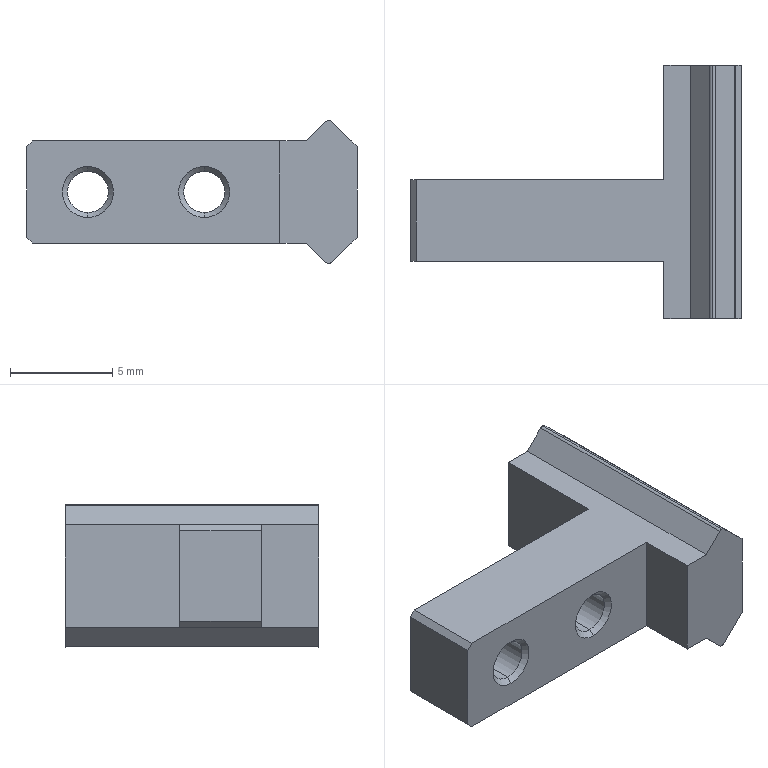Part | SolidWorks | features BaseBody 1 | 1 solid | 35 faces | box 16.2 x 12.4 x 6.994 mm | volume 484.765 mm3 | plane 20 | cone 8 | cylinder 7 | commonest cylinder face diameters 2.013 x4 0.4 x3
STEP:
#1=CARTESIAN_POINT('',(-42.341,-14.4,3.439));
#2=VERTEX_POINT('',#1);
#3=CARTESIAN_POINT('',(-42.2,-14.4,3.497));
#4=VERTEX_POINT('',#3);
#5=CARTESIAN_POINT('',(-42.2,-14.4,3.297));
#6=DIRECTION('',(0.,1.,0.));
#7=DIRECTION('',(1.,0.,0.));
#8=AXIS2_PLACEMENT_3D('',#5,#6,#7);
#9=CIRCLE('',#8,0.2);
#10=EDGE_CURVE('',#2,#4,#9,.T.);
#11=ORIENTED_EDGE('',*,*,#10,.T.);
#12=CARTESIAN_POINT('',(-42.2,-2.,3.497));
#13=VERTEX_POINT('',#12);
#14=CARTESIAN_POINT('',(-42.2,-14.4,3.497));
#15=DIRECTION('',(0.,1.,0.));
#16=VECTOR('',#15,1000.);
#17=LINE('',#14,#16);
#18=EDGE_CURVE('',#4,#13,#17,.T.);
#19=ORIENTED_EDGE('',*,*,#18,.T.);
#20=CARTESIAN_POINT('',(-42.341,-2.,3.439));
#21=VERTEX_POINT('',#20);
#22=CARTESIAN_POINT('',(-42.2,-2.,3.297));
#23=DIRECTION('',(0.,1.,0.));
#24=DIRECTION('',(1.,0.,0.));
#25=AXIS2_PLACEMENT_3D('',#22,#23,#24);
#26=CIRCLE('',#25,0.2);
#27=EDGE_CURVE('',#21,#13,#26,.T.);
#28=ORIENTED_EDGE('',*,*,#27,.F.);
#29=CARTESIAN_POINT('',(-42.341,-14.4,3.439));
#30=DIRECTION('',(0.,1.,0.));
#31=VECTOR('',#30,1000.);
#32=LINE('',#29,#31);
#33=EDGE_CURVE('',#2,#21,#32,.T.);
#34=ORIENTED_EDGE('',*,*,#33,.F.);
#35=EDGE_LOOP('',(#11,#19,#28,#34));
#36=FACE_OUTER_BOUND('',#35,.T.);
#37=CARTESIAN_POINT('',(-42.2,-14.4,3.297));
#38=DIRECTION('',(0.,1.,0.));
#39=DIRECTION('',(0.,0.,1.));
#40=AXIS2_PLACEMENT_3D('',#37,#38,#39);
#41=CYLINDRICAL_SURFACE('',#40,0.2);
#42=ADVANCED_FACE('',(#36),#41,.T.);
#43=CARTESIAN_POINT('',(-54.,-11.357,-1.006));
#44=VERTEX_POINT('',#43);
#45=CARTESIAN_POINT('',(-54.,-11.357,1.006));
#46=VERTEX_POINT('',#45);
#47=CARTESIAN_POINT('',(-54.,-11.357,0.));
#48=DIRECTION('',(0.,1.,0.));
#49=DIRECTION('',(0.,0.,1.));
#50=AXIS2_PLACEMENT_3D('',#47,#48,#49);
#51=CIRCLE('',#50,1.006);
#52=EDGE_CURVE('',#44,#46,#51,.T.);
#53=ORIENTED_EDGE('',*,*,#52,.T.);
#54=CARTESIAN_POINT('',(-54.,-11.6,1.25));
#55=VERTEX_POINT('',#54);
#56=CARTESIAN_POINT('',(-54.,-11.6,1.25));
#57=DIRECTION('',(0.,-0.7071,0.7071));
#58=VECTOR('',#57,1000.);
#59=LINE('',#56,#58);
#60=EDGE_CURVE('',#46,#55,#59,.T.);
#61=ORIENTED_EDGE('',*,*,#60,.T.);
#62=CARTESIAN_POINT('',(-54.,-11.6,-1.25));
#63=VERTEX_POINT('',#62);
#64=CARTESIAN_POINT('',(-54.,-11.6,0.));
#65=DIRECTION('',(0.,1.,0.));
#66=DIRECTION('',(0.,0.,1.));
#67=AXIS2_PLACEMENT_3D('',#64,#65,#66);
#68=CIRCLE('',#67,1.25);
#69=EDGE_CURVE('',#63,#55,#68,.T.);
#70=ORIENTED_EDGE('',*,*,#69,.F.);
#71=CARTESIAN_POINT('',(-54.,-11.6,-1.25));
#72=DIRECTION('',(0.,-0.7071,-0.7071));
#73=VECTOR('',#72,1000.);
#74=LINE('',#71,#73);
#75=EDGE_CURVE('',#44,#63,#74,.T.);
#76=ORIENTED_EDGE('',*,*,#75,.F.);
#77=EDGE_LOOP('',(#53,#61,#70,#76));
#78=FACE_OUTER_BOUND('',#77,.T.);
#79=CARTESIAN_POINT('',(-54.,-11.6,0.));
#80=DIRECTION('',(0.,-1.,0.));
#81=DIRECTION('',(0.,0.,-1.));
#82=AXIS2_PLACEMENT_3D('',#79,#80,#81);
#83=CONICAL_SURFACE('',#82,1.25,0.7854);
#84=ADVANCED_FACE('',(#78),#83,.F.);
#85=ORIENTED_EDGE('',*,*,#52,.F.);
#86=CARTESIAN_POINT('',(-54.,-7.833,-1.006));
#87=VERTEX_POINT('',#86);
#88=CARTESIAN_POINT('',(-54.,-7.59,-1.006));
#89=DIRECTION('',(0.,1.,0.));
#90=VECTOR('',#89,1000.);
#91=LINE('',#88,#90);
#92=EDGE_CURVE('',#44,#87,#91,.T.);
#93=ORIENTED_EDGE('',*,*,#92,.T.);
#94=CARTESIAN_POINT('',(-54.,-7.833,1.006));
#95=VERTEX_POINT('',#94);
#96=CARTESIAN_POINT('',(-54.,-7.833,0.));
#97=DIRECTION('',(0.,1.,0.));
#98=DIRECTION('',(0.,0.,1.));
#99=AXIS2_PLACEMENT_3D('',#96,#97,#98);
#100=CIRCLE('',#99,1.006);
#101=EDGE_CURVE('',#87,#95,#100,.T.);
#102=ORIENTED_EDGE('',*,*,#101,.T.);
#103=CARTESIAN_POINT('',(-54.,-7.59,1.006));
#104=DIRECTION('',(0.,1.,0.));
#105=VECTOR('',#104,1000.);
#106=LINE('',#103,#105);
#107=EDGE_CURVE('',#46,#95,#106,.T.);
#108=ORIENTED_EDGE('',*,*,#107,.F.);
#109=EDGE_LOOP('',(#85,#93,#102,#108));
#110=FACE_OUTER_BOUND('',#109,.T.);
#111=CARTESIAN_POINT('',(-54.,-7.59,0.));
#112=DIRECTION('',(0.,1.,0.));
#113=DIRECTION('',(0.,0.,1.));
#114=AXIS2_PLACEMENT_3D('',#111,#112,#113);
#115=CYLINDRICAL_SURFACE('',#114,1.006);
#116=ADVANCED_FACE('',(#110),#115,.F.);
#117=ORIENTED_EDGE('',*,*,#101,.F.);
#118=CARTESIAN_POINT('',(-54.,-7.6,-1.24));
#119=VERTEX_POINT('',#118);
#120=CARTESIAN_POINT('',(-54.,-7.833,-1.006));
#121=DIRECTION('',(0.,0.7071,-0.7071));
#122=VECTOR('',#121,1000.);
#123=LINE('',#120,#122);
#124=EDGE_CURVE('',#87,#119,#123,.T.);
#125=ORIENTED_EDGE('',*,*,#124,.T.);
#126=CARTESIAN_POINT('',(-54.,-7.6,1.24));
#127=VERTEX_POINT('',#126);
#128=CARTESIAN_POINT('',(-54.,-7.6,0.));
#129=DIRECTION('',(0.,-1.,0.));
#130=DIRECTION('',(0.,0.,1.));
#131=AXIS2_PLACEMENT_3D('',#128,#129,#130);
#132=CIRCLE('',#131,1.24);
#133=EDGE_CURVE('',#127,#119,#132,.T.);
#134=ORIENTED_EDGE('',*,*,#133,.F.);
#135=CARTESIAN_POINT('',(-54.,-7.833,1.006));
#136=DIRECTION('',(0.,0.7071,0.7071));
#137=VECTOR('',#136,1000.);
#138=LINE('',#135,#137);
#139=EDGE_CURVE('',#95,#127,#138,.T.);
#140=ORIENTED_EDGE('',*,*,#139,.F.);
#141=EDGE_LOOP('',(#117,#125,#134,#140));
#142=FACE_OUTER_BOUND('',#141,.T.);
#143=CARTESIAN_POINT('',(-54.,-7.833,0.));
#144=DIRECTION('',(0.,1.,0.));
#145=DIRECTION('',(0.,0.,1.));
#146=AXIS2_PLACEMENT_3D('',#143,#144,#145);
#147=CONICAL_SURFACE('',#146,1.006,0.7854);
#148=ADVANCED_FACE('',(#142),#147,.F.);
#149=CARTESIAN_POINT('',(-48.3,-11.357,-1.006));
#150=VERTEX_POINT('',#149);
#151=CARTESIAN_POINT('',(-48.3,-11.357,1.006));
#152=VERTEX_POINT('',#151);
#153=CARTESIAN_POINT('',(-48.3,-11.357,0.));
#154=DIRECTION('',(0.,1.,0.));
#155=DIRECTION('',(0.,0.,1.));
#156=AXIS2_PLACEMENT_3D('',#153,#154,#155);
#157=CIRCLE('',#156,1.006);
#158=EDGE_CURVE('',#150,#152,#157,.T.);
#159=ORIENTED_EDGE('',*,*,#158,.T.);
#160=CARTESIAN_POINT('',(-48.3,-11.6,1.25));
#161=VERTEX_POINT('',#160);
#162=CARTESIAN_POINT('',(-48.3,-11.6,1.25));
#163=DIRECTION('',(0.,-0.7071,0.7071));
#164=VECTOR('',#163,1000.);
#165=LINE('',#162,#164);
#166=EDGE_CURVE('',#152,#161,#165,.T.);
#167=ORIENTED_EDGE('',*,*,#166,.T.);
#168=CARTESIAN_POINT('',(-48.3,-11.6,-1.25));
#169=VERTEX_POINT('',#168);
#170=CARTESIAN_POINT('',(-48.3,-11.6,0.));
#171=DIRECTION('',(0.,1.,0.));
#172=DIRECTION('',(0.,0.,1.));
#173=AXIS2_PLACEMENT_3D('',#170,#171,#172);
#174=CIRCLE('',#173,1.25);
#175=EDGE_CURVE('',#169,#161,#174,.T.);
#176=ORIENTED_EDGE('',*,*,#175,.F.);
#177=CARTESIAN_POINT('',(-48.3,-11.6,-1.25));
#178=DIRECTION('',(0.,-0.7071,-0.7071));
#179=VECTOR('',#178,1000.);
#180=LINE('',#177,#179);
#181=EDGE_CURVE('',#150,#169,#180,.T.);
#182=ORIENTED_EDGE('',*,*,#181,.F.);
#183=EDGE_LOOP('',(#159,#167,#176,#182));
#184=FACE_OUTER_BOUND('',#183,.T.);
#185=CARTESIAN_POINT('',(-48.3,-11.6,0.));
#186=DIRECTION('',(0.,-1.,0.));
#187=DIRECTION('',(0.,0.,-1.));
#188=AXIS2_PLACEMENT_3D('',#185,#186,#187);
#189=CONICAL_SURFACE('',#188,1.25,0.7854);
#190=ADVANCED_FACE('',(#184),#189,.F.);
#191=ORIENTED_EDGE('',*,*,#158,.F.);
#192=CARTESIAN_POINT('',(-48.3,-7.833,-1.006));
#193=VERTEX_POINT('',#192);
#194=CARTESIAN_POINT('',(-48.3,-7.59,-1.006));
#195=DIRECTION('',(0.,1.,0.));
#196=VECTOR('',#195,1000.);
#197=LINE('',#194,#196);
#198=EDGE_CURVE('',#150,#193,#197,.T.);
#199=ORIENTED_EDGE('',*,*,#198,.T.);
#200=CARTESIAN_POINT('',(-48.3,-7.833,1.006));
#201=VERTEX_POINT('',#200);
#202=CARTESIAN_POINT('',(-48.3,-7.833,0.));
#203=DIRECTION('',(0.,1.,0.));
#204=DIRECTION('',(0.,0.,1.));
#205=AXIS2_PLACEMENT_3D('',#202,#203,#204);
#206=CIRCLE('',#205,1.006);
#207=EDGE_CURVE('',#193,#201,#206,.T.);
#208=ORIENTED_EDGE('',*,*,#207,.T.);
#209=CARTESIAN_POINT('',(-48.3,-7.59,1.006));
#210=DIRECTION('',(0.,1.,0.));
#211=VECTOR('',#210,1000.);
#212=LINE('',#209,#211);
#213=EDGE_CURVE('',#152,#201,#212,.T.);
#214=ORIENTED_EDGE('',*,*,#213,.F.);
#215=EDGE_LOOP('',(#191,#199,#208,#214));
#216=FACE_OUTER_BOUND('',#215,.T.);
#217=CARTESIAN_POINT('',(-48.3,-7.59,0.));
#218=DIRECTION('',(0.,1.,0.));
#219=DIRECTION('',(0.,0.,1.));
#220=AXIS2_PLACEMENT_3D('',#217,#218,#219);
#221=CYLINDRICAL_SURFACE('',#220,1.006);
#222=ADVANCED_FACE('',(#216),#221,.F.);
#223=ORIENTED_EDGE('',*,*,#207,.F.);
#224=CARTESIAN_POINT('',(-48.3,-7.6,-1.24));
#225=VERTEX_POINT('',#224);
#226=CARTESIAN_POINT('',(-48.3,-7.833,-1.006));
#227=DIRECTION('',(0.,0.7071,-0.7071));
#228=VECTOR('',#227,1000.);
#229=LINE('',#226,#228);
#230=EDGE_CURVE('',#193,#225,#229,.T.);
#231=ORIENTED_EDGE('',*,*,#230,.T.);
#232=CARTESIAN_POINT('',(-48.3,-7.6,1.24));
#233=VERTEX_POINT('',#232);
#234=CARTESIAN_POINT('',(-48.3,-7.6,0.));
#235=DIRECTION('',(0.,-1.,0.));
#236=DIRECTION('',(0.,0.,1.));
#237=AXIS2_PLACEMENT_3D('',#234,#235,#236);
#238=CIRCLE('',#237,1.24);
#239=EDGE_CURVE('',#233,#225,#238,.T.);
#240=ORIENTED_EDGE('',*,*,#239,.F.);
#241=CARTESIAN_POINT('',(-48.3,-7.833,1.006));
#242=DIRECTION('',(0.,0.7071,0.7071));
#243=VECTOR('',#242,1000.);
#244=LINE('',#241,#243);
#245=EDGE_CURVE('',#201,#233,#244,.T.);
#246=ORIENTED_EDGE('',*,*,#245,.F.);
#247=EDGE_LOOP('',(#223,#231,#240,#246));
#248=FACE_OUTER_BOUND('',#247,.T.);
#249=CARTESIAN_POINT('',(-48.3,-7.833,0.));
#250=DIRECTION('',(0.,1.,0.));
#251=DIRECTION('',(0.,0.,1.));
#252=AXIS2_PLACEMENT_3D('',#249,#250,#251);
#253=CONICAL_SURFACE('',#252,1.006,0.7854);
#254=ADVANCED_FACE('',(#248),#253,.F.);
#255=ORIENTED_EDGE('',*,*,#230,.F.);
#256=CARTESIAN_POINT('',(-48.3,-7.833,0.));
#257=DIRECTION('',(0.,1.,0.));
#258=DIRECTION('',(0.,0.,1.));
#259=AXIS2_PLACEMENT_3D('',#256,#257,#258);
#260=CIRCLE('',#259,1.006);
#261=EDGE_CURVE('',#201,#193,#260,.T.);
#262=ORIENTED_EDGE('',*,*,#261,.F.);
#263=ORIENTED_EDGE('',*,*,#245,.T.);
#264=CARTESIAN_POINT('',(-48.3,-7.6,0.));
#265=DIRECTION('',(0.,-1.,0.));
#266=DIRECTION('',(0.,0.,1.));
#267=AXIS2_PLACEMENT_3D('',#264,#265,#266);
#268=CIRCLE('',#267,1.24);
#269=EDGE_CURVE('',#225,#233,#268,.T.);
#270=ORIENTED_EDGE('',*,*,#269,.F.);
#271=EDGE_LOOP('',(#255,#262,#263,#270));
#272=FACE_OUTER_BOUND('',#271,.T.);
#273=CARTESIAN_POINT('',(-48.3,-7.833,0.));
#274=DIRECTION('',(0.,1.,0.));
#275=DIRECTION('',(0.,0.,1.));
#276=AXIS2_PLACEMENT_3D('',#273,#274,#275);
#277=CONICAL_SURFACE('',#276,1.006,0.7854);
#278=ADVANCED_FACE('',(#272),#277,.F.);
#279=ORIENTED_EDGE('',*,*,#198,.F.);
#280=CARTESIAN_POINT('',(-48.3,-11.357,0.));
#281=DIRECTION('',(0.,1.,0.));
#282=DIRECTION('',(0.,0.,1.));
#283=AXIS2_PLACEMENT_3D('',#280,#281,#282);
#284=CIRCLE('',#283,1.006);
#285=EDGE_CURVE('',#152,#150,#284,.T.);
#286=ORIENTED_EDGE('',*,*,#285,.F.);
#287=ORIENTED_EDGE('',*,*,#213,.T.);
#288=ORIENTED_EDGE('',*,*,#261,.T.);
#289=EDGE_LOOP('',(#279,#286,#287,#288));
#290=FACE_OUTER_BOUND('',#289,.T.);
#291=CARTESIAN_POINT('',(-48.3,-7.59,0.));
#292=DIRECTION('',(0.,1.,0.));
#293=DIRECTION('',(0.,0.,1.));
#294=AXIS2_PLACEMENT_3D('',#291,#292,#293);
#295=CYLINDRICAL_SURFACE('',#294,1.006);
#296=ADVANCED_FACE('',(#290),#295,.F.);
#297=ORIENTED_EDGE('',*,*,#166,.F.);
#298=ORIENTED_EDGE('',*,*,#285,.T.);
#299=ORIENTED_EDGE('',*,*,#181,.T.);
#300=CARTESIAN_POINT('',(-48.3,-11.6,0.));
#301=DIRECTION('',(0.,1.,0.));
#302=DIRECTION('',(0.,0.,1.));
#303=AXIS2_PLACEMENT_3D('',#300,#301,#302);
#304=CIRCLE('',#303,1.25);
#305=EDGE_CURVE('',#161,#169,#304,.T.);
#306=ORIENTED_EDGE('',*,*,#305,.F.);
#307=EDGE_LOOP('',(#297,#298,#299,#306));
#308=FACE_OUTER_BOUND('',#307,.T.);
#309=CARTESIAN_POINT('',(-48.3,-11.6,0.));
#310=DIRECTION('',(0.,-1.,0.));
#311=DIRECTION('',(0.,0.,-1.));
#312=AXIS2_PLACEMENT_3D('',#309,#310,#311);
#313=CONICAL_SURFACE('',#312,1.25,0.7854);
#314=ADVANCED_FACE('',(#308),#313,.F.);
#315=ORIENTED_EDGE('',*,*,#124,.F.);
#316=CARTESIAN_POINT('',(-54.,-7.833,0.));
#317=DIRECTION('',(0.,1.,0.));
#318=DIRECTION('',(0.,0.,1.));
#319=AXIS2_PLACEMENT_3D('',#316,#317,#318);
#320=CIRCLE('',#319,1.006);
#321=EDGE_CURVE('',#95,#87,#320,.T.);
#322=ORIENTED_EDGE('',*,*,#321,.F.);
#323=ORIENTED_EDGE('',*,*,#139,.T.);
#324=CARTESIAN_POINT('',(-54.,-7.6,0.));
#325=DIRECTION('',(0.,-1.,0.));
#326=DIRECTION('',(0.,0.,1.));
#327=AXIS2_PLACEMENT_3D('',#324,#325,#326);
#328=CIRCLE('',#327,1.24);
#329=EDGE_CURVE('',#119,#127,#328,.T.);
#330=ORIENTED_EDGE('',*,*,#329,.F.);
#331=EDGE_LOOP('',(#315,#322,#323,#330));
#332=FACE_OUTER_BOUND('',#331,.T.);
#333=CARTESIAN_POINT('',(-54.,-7.833,0.));
#334=DIRECTION('',(0.,1.,0.));
#335=DIRECTION('',(0.,0.,1.));
#336=AXIS2_PLACEMENT_3D('',#333,#334,#335);
#337=CONICAL_SURFACE('',#336,1.006,0.7854);
#338=ADVANCED_FACE('',(#332),#337,.F.);
#339=ORIENTED_EDGE('',*,*,#92,.F.);
#340=CARTESIAN_POINT('',(-54.,-11.357,0.));
#341=DIRECTION('',(0.,1.,0.));
#342=DIRECTION('',(0.,0.,1.));
#343=AXIS2_PLACEMENT_3D('',#340,#341,#342);
#344=CIRCLE('',#343,1.006);
#345=EDGE_CURVE('',#46,#44,#344,.T.);
#346=ORIENTED_EDGE('',*,*,#345,.F.);
#347=ORIENTED_EDGE('',*,*,#107,.T.);
#348=ORIENTED_EDGE('',*,*,#321,.T.);
#349=EDGE_LOOP('',(#339,#346,#347,#348));
#350=FACE_OUTER_BOUND('',#349,.T.);
#351=CARTESIAN_POINT('',(-54.,-7.59,0.));
#352=DIRECTION('',(0.,1.,0.));
#353=DIRECTION('',(0.,0.,1.));
#354=AXIS2_PLACEMENT_3D('',#351,#352,#353);
#355=CYLINDRICAL_SURFACE('',#354,1.006);
#356=ADVANCED_FACE('',(#350),#355,.F.);
#357=ORIENTED_EDGE('',*,*,#60,.F.);
#358=ORIENTED_EDGE('',*,*,#345,.T.);
#359=ORIENTED_EDGE('',*,*,#75,.T.);
#360=CARTESIAN_POINT('',(-54.,-11.6,0.));
#361=DIRECTION('',(0.,1.,0.));
#362=DIRECTION('',(0.,0.,1.));
#363=AXIS2_PLACEMENT_3D('',#360,#361,#362);
#364=CIRCLE('',#363,1.25);
#365=EDGE_CURVE('',#55,#63,#364,.T.);
#366=ORIENTED_EDGE('',*,*,#365,.F.);
#367=EDGE_LOOP('',(#357,#358,#359,#366));
#368=FACE_OUTER_BOUND('',#367,.T.);
#369=CARTESIAN_POINT('',(-54.,-11.6,0.));
#370=DIRECTION('',(0.,-1.,0.));
#371=DIRECTION('',(0.,0.,-1.));
#372=AXIS2_PLACEMENT_3D('',#369,#370,#371);
#373=CONICAL_SURFACE('',#372,1.25,0.7854);
#374=ADVANCED_FACE('',(#368),#373,.F.);
#375=CARTESIAN_POINT('',(-57.,-7.6,-2.217));
#376=VERTEX_POINT('',#375);
#377=CARTESIAN_POINT('',(-57.,-7.6,2.217));
#378=VERTEX_POINT('',#377);
#379=CARTESIAN_POINT('',(-57.,-7.6,-2.217));
#380=DIRECTION('',(0.,0.,1.));
#381=VECTOR('',#380,1000.);
#382=LINE('',#379,#381);
#383=EDGE_CURVE('',#376,#378,#382,.T.);
#384=ORIENTED_EDGE('',*,*,#383,.T.);
#385=CARTESIAN_POINT('',(-56.717,-7.6,2.5));
#386=VERTEX_POINT('',#385);
#387=CARTESIAN_POINT('',(-57.,-7.6,2.217));
#388=DIRECTION('',(0.7071,0.,0.7071));
#389=VECTOR('',#388,1000.);
#390=LINE('',#387,#389);
#391=EDGE_CURVE('',#378,#386,#390,.T.);
#392=ORIENTED_EDGE('',*,*,#391,.T.);
#393=CARTESIAN_POINT('',(-44.6,-7.6,2.5));
#394=VERTEX_POINT('',#393);
#395=CARTESIAN_POINT('',(-56.717,-7.6,2.5));
#396=DIRECTION('',(1.,0.,0.));
#397=VECTOR('',#396,1000.);
#398=LINE('',#395,#397);
#399=EDGE_CURVE('',#386,#394,#398,.T.);
#400=ORIENTED_EDGE('',*,*,#399,.T.);
#401=CARTESIAN_POINT('',(-44.6,-7.6,-2.5));
#402=VERTEX_POINT('',#401);
#403=CARTESIAN_POINT('',(-44.6,-7.6,2.5));
#404=DIRECTION('',(0.,0.,-1.));
#405=VECTOR('',#404,1000.);
#406=LINE('',#403,#405);
#407=EDGE_CURVE('',#394,#402,#406,.T.);
#408=ORIENTED_EDGE('',*,*,#407,.T.);
#409=CARTESIAN_POINT('',(-56.717,-7.6,-2.5));
#410=VERTEX_POINT('',#409);
#411=CARTESIAN_POINT('',(-44.6,-7.6,-2.5));
#412=DIRECTION('',(-1.,0.,0.));
#413=VECTOR('',#412,1000.);
#414=LINE('',#411,#413);
#415=EDGE_CURVE('',#402,#410,#414,.T.);
#416=ORIENTED_EDGE('',*,*,#415,.T.);
#417=CARTESIAN_POINT('',(-56.717,-7.6,-2.5));
#418=DIRECTION('',(-0.7071,0.,0.7071));
#419=VECTOR('',#418,1000.);
#420=LINE('',#417,#419);
#421=EDGE_CURVE('',#410,#376,#420,.T.);
#422=ORIENTED_EDGE('',*,*,#421,.T.);
#423=EDGE_LOOP('',(#384,#392,#400,#408,#416,#422));
#424=FACE_OUTER_BOUND('',#423,.T.);
#425=ORIENTED_EDGE('',*,*,#133,.T.);
#426=ORIENTED_EDGE('',*,*,#329,.T.);
#427=EDGE_LOOP('',(#425,#426));
#428=FACE_BOUND('',#427,.T.);
#429=ORIENTED_EDGE('',*,*,#239,.T.);
#430=ORIENTED_EDGE('',*,*,#269,.T.);
#431=EDGE_LOOP('',(#429,#430));
#432=FACE_BOUND('',#431,.T.);
#433=CARTESIAN_POINT('',(0.,-7.6,0.));
#434=DIRECTION('',(0.,1.,0.));
#435=DIRECTION('',(1.,0.,0.));
#436=AXIS2_PLACEMENT_3D('',#433,#434,#435);
#437=PLANE('',#436);
#438=ADVANCED_FACE('',(#424,#428,#432),#437,.T.);
#439=CARTESIAN_POINT('',(-57.,-11.6,-2.217));
#440=VERTEX_POINT('',#439);
#441=CARTESIAN_POINT('',(-57.,-11.6,2.217));
#442=VERTEX_POINT('',#441);
#443=CARTESIAN_POINT('',(-57.,-11.6,-2.217));
#444=DIRECTION('',(0.,0.,1.));
#445=VECTOR('',#444,1000.);
#446=LINE('',#443,#445);
#447=EDGE_CURVE('',#440,#442,#446,.T.);
#448=ORIENTED_EDGE('',*,*,#447,.F.);
#449=CARTESIAN_POINT('',(-56.717,-11.6,-2.5));
#450=VERTEX_POINT('',#449);
#451=CARTESIAN_POINT('',(-56.717,-11.6,-2.5));
#452=DIRECTION('',(-0.7071,0.,0.7071));
#453=VECTOR('',#452,1000.);
#454=LINE('',#451,#453);
#455=EDGE_CURVE('',#450,#440,#454,.T.);
#456=ORIENTED_EDGE('',*,*,#455,.F.);
#457=CARTESIAN_POINT('',(-44.6,-11.6,-2.5));
#458=VERTEX_POINT('',#457);
#459=CARTESIAN_POINT('',(-44.6,-11.6,-2.5));
#460=DIRECTION('',(-1.,0.,0.));
#461=VECTOR('',#460,1000.);
#462=LINE('',#459,#461);
#463=EDGE_CURVE('',#458,#450,#462,.T.);
#464=ORIENTED_EDGE('',*,*,#463,.F.);
#465=CARTESIAN_POINT('',(-44.6,-11.6,2.5));
#466=VERTEX_POINT('',#465);
#467=CARTESIAN_POINT('',(-44.6,-11.6,2.5));
#468=DIRECTION('',(0.,0.,-1.));
#469=VECTOR('',#468,1000.);
#470=LINE('',#467,#469);
#471=EDGE_CURVE('',#466,#458,#470,.T.);
#472=ORIENTED_EDGE('',*,*,#471,.F.);
#473=CARTESIAN_POINT('',(-56.717,-11.6,2.5));
#474=VERTEX_POINT('',#473);
#475=CARTESIAN_POINT('',(-56.717,-11.6,2.5));
#476=DIRECTION('',(1.,0.,0.));
#477=VECTOR('',#476,1000.);
#478=LINE('',#475,#477);
#479=EDGE_CURVE('',#474,#466,#478,.T.);
#480=ORIENTED_EDGE('',*,*,#479,.F.);
#481=CARTESIAN_POINT('',(-57.,-11.6,2.217));
#482=DIRECTION('',(0.7071,0.,0.7071));
#483=VECTOR('',#482,1000.);
#484=LINE('',#481,#483);
#485=EDGE_CURVE('',#442,#474,#484,.T.);
#486=ORIENTED_EDGE('',*,*,#485,.F.);
#487=EDGE_LOOP('',(#448,#456,#464,#472,#480,#486));
#488=FACE_OUTER_BOUND('',#487,.T.);
#489=ORIENTED_EDGE('',*,*,#69,.T.);
#490=ORIENTED_EDGE('',*,*,#365,.T.);
#491=EDGE_LOOP('',(#489,#490));
#492=FACE_BOUND('',#491,.T.);
#493=ORIENTED_EDGE('',*,*,#175,.T.);
#494=ORIENTED_EDGE('',*,*,#305,.T.);
#495=EDGE_LOOP('',(#493,#494));
#496=FACE_BOUND('',#495,.T.);
#497=CARTESIAN_POINT('',(0.,-11.6,0.));
#498=DIRECTION('',(0.,1.,0.));
#499=DIRECTION('',(1.,0.,0.));
#500=AXIS2_PLACEMENT_3D('',#497,#498,#499);
#501=PLANE('',#500);
#502=ADVANCED_FACE('',(#488,#492,#496),#501,.F.);
#503=ORIENTED_EDGE('',*,*,#421,.F.);
#504=CARTESIAN_POINT('',(-56.717,-11.6,-2.5));
#505=DIRECTION('',(0.,1.,0.));
#506=VECTOR('',#505,1000.);
#507=LINE('',#504,#506);
#508=EDGE_CURVE('',#450,#410,#507,.T.);
#509=ORIENTED_EDGE('',*,*,#508,.F.);
#510=ORIENTED_EDGE('',*,*,#455,.T.);
#511=CARTESIAN_POINT('',(-57.,-11.6,-2.217));
#512=DIRECTION('',(0.,1.,0.));
#513=VECTOR('',#512,1000.);
#514=LINE('',#511,#513);
#515=EDGE_CURVE('',#440,#376,#514,.T.);
#516=ORIENTED_EDGE('',*,*,#515,.T.);
#517=EDGE_LOOP('',(#503,#509,#510,#516));
#518=FACE_OUTER_BOUND('',#517,.T.);
#519=CARTESIAN_POINT('',(-56.717,-11.6,-2.5));
#520=DIRECTION('',(-0.7071,0.,-0.7071));
#521=DIRECTION('',(-0.7071,0.,0.7071));
#522=AXIS2_PLACEMENT_3D('',#519,#520,#521);
#523=PLANE('',#522);
#524=ADVANCED_FACE('',(#518),#523,.T.);
#525=ORIENTED_EDGE('',*,*,#391,.F.);
#526=CARTESIAN_POINT('',(-57.,-11.6,2.217));
#527=DIRECTION('',(0.,1.,0.));
#528=VECTOR('',#527,1000.);
#529=LINE('',#526,#528);
#530=EDGE_CURVE('',#442,#378,#529,.T.);
#531=ORIENTED_EDGE('',*,*,#530,.F.);
#532=ORIENTED_EDGE('',*,*,#485,.T.);
#533=CARTESIAN_POINT('',(-56.717,-11.6,2.5));
#534=DIRECTION('',(0.,1.,0.));
#535=VECTOR('',#534,1000.);
#536=LINE('',#533,#535);
#537=EDGE_CURVE('',#474,#386,#536,.T.);
#538=ORIENTED_EDGE('',*,*,#537,.T.);
#539=EDGE_LOOP('',(#525,#531,#532,#538));
#540=FACE_OUTER_BOUND('',#539,.T.);
#541=CARTESIAN_POINT('',(-57.,-11.6,2.217));
#542=DIRECTION('',(-0.7071,0.,0.7071));
#543=DIRECTION('',(0.,1.,0.));
#544=AXIS2_PLACEMENT_3D('',#541,#542,#543);
#545=PLANE('',#544);
#546=ADVANCED_FACE('',(#540),#545,.T.);
#547=ORIENTED_EDGE('',*,*,#383,.F.);
#548=ORIENTED_EDGE('',*,*,#515,.F.);
#549=ORIENTED_EDGE('',*,*,#447,.T.);
#550=ORIENTED_EDGE('',*,*,#530,.T.);
#551=EDGE_LOOP('',(#547,#548,#549,#550));
#552=FACE_OUTER_BOUND('',#551,.T.);
#553=CARTESIAN_POINT('',(-57.,-11.6,-2.217));
#554=DIRECTION('',(-1.,0.,0.));
#555=DIRECTION('',(0.,0.,1.));
#556=AXIS2_PLACEMENT_3D('',#553,#554,#555);
#557=PLANE('',#556);
#558=ADVANCED_FACE('',(#552),#557,.T.);
#559=CARTESIAN_POINT('',(-43.28,-2.,-2.5));
#560=VERTEX_POINT('',#559);
#561=CARTESIAN_POINT('',(-44.6,-2.,-2.5));
#562=VERTEX_POINT('',#561);
#563=CARTESIAN_POINT('',(-43.28,-2.,-2.5));
#564=DIRECTION('',(-1.,0.,0.));
#565=VECTOR('',#564,1000.);
#566=LINE('',#563,#565);
#567=EDGE_CURVE('',#560,#562,#566,.T.);
#568=ORIENTED_EDGE('',*,*,#567,.T.);
#569=CARTESIAN_POINT('',(-44.6,-2.,2.5));
#570=VERTEX_POINT('',#569);
#571=CARTESIAN_POINT('',(-44.6,-2.,-2.5));
#572=DIRECTION('',(0.,0.,1.));
#573=VECTOR('',#572,1000.);
#574=LINE('',#571,#573);
#575=EDGE_CURVE('',#562,#570,#574,.T.);
#576=ORIENTED_EDGE('',*,*,#575,.T.);
#577=CARTESIAN_POINT('',(-43.28,-2.,2.5));
#578=VERTEX_POINT('',#577);
#579=CARTESIAN_POINT('',(-44.6,-2.,2.5));
#580=DIRECTION('',(1.,0.,0.));
#581=VECTOR('',#580,1000.);
#582=LINE('',#579,#581);
#583=EDGE_CURVE('',#570,#578,#582,.T.);
#584=ORIENTED_EDGE('',*,*,#583,.T.);
#585=CARTESIAN_POINT('',(-43.28,-2.,2.5));
#586=DIRECTION('',(0.7071,0.,0.7071));
#587=VECTOR('',#586,1000.);
#588=LINE('',#585,#587);
#589=EDGE_CURVE('',#578,#21,#588,.T.);
#590=ORIENTED_EDGE('',*,*,#589,.T.);
#591=ORIENTED_EDGE('',*,*,#27,.T.);
#592=CARTESIAN_POINT('',(-42.059,-2.,3.439));
#593=VERTEX_POINT('',#592);
#594=CARTESIAN_POINT('',(-42.2,-2.,3.297));
#595=DIRECTION('',(0.,1.,0.));
#596=DIRECTION('',(1.,0.,0.));
#597=AXIS2_PLACEMENT_3D('',#594,#595,#596);
#598=CIRCLE('',#597,0.2);
#599=EDGE_CURVE('',#13,#593,#598,.T.);
#600=ORIENTED_EDGE('',*,*,#599,.T.);
#601=CARTESIAN_POINT('',(-41.12,-2.,2.5));
#602=VERTEX_POINT('',#601);
#603=CARTESIAN_POINT('',(-42.059,-2.,3.439));
#604=DIRECTION('',(0.7071,0.,-0.7071));
#605=VECTOR('',#604,1000.);
#606=LINE('',#603,#605);
#607=EDGE_CURVE('',#593,#602,#606,.T.);
#608=ORIENTED_EDGE('',*,*,#607,.T.);
#609=CARTESIAN_POINT('',(-41.083,-2.,2.5));
#610=VERTEX_POINT('',#609);
#611=CARTESIAN_POINT('',(-41.12,-2.,2.5));
#612=DIRECTION('',(1.,0.,0.));
#613=VECTOR('',#612,1000.);
#614=LINE('',#611,#613);
#615=EDGE_CURVE('',#602,#610,#614,.T.);
#616=ORIENTED_EDGE('',*,*,#615,.T.);
#617=CARTESIAN_POINT('',(-40.8,-2.,2.217));
#618=VERTEX_POINT('',#617);
#619=CARTESIAN_POINT('',(-41.083,-2.,2.5));
#620=DIRECTION('',(0.7071,0.,-0.7071));
#621=VECTOR('',#620,1000.);
#622=LINE('',#619,#621);
#623=EDGE_CURVE('',#610,#618,#622,.T.);
#624=ORIENTED_EDGE('',*,*,#623,.T.);
#625=CARTESIAN_POINT('',(-40.8,-2.,-2.217));
#626=VERTEX_POINT('',#625);
#627=CARTESIAN_POINT('',(-40.8,-2.,2.217));
#628=DIRECTION('',(0.,0.,-1.));
#629=VECTOR('',#628,1000.);
#630=LINE('',#627,#629);
#631=EDGE_CURVE('',#618,#626,#630,.T.);
#632=ORIENTED_EDGE('',*,*,#631,.T.);
#633=CARTESIAN_POINT('',(-41.083,-2.,-2.5));
#634=VERTEX_POINT('',#633);
#635=CARTESIAN_POINT('',(-40.8,-2.,-2.217));
#636=DIRECTION('',(-0.7071,0.,-0.7071));
#637=VECTOR('',#636,1000.);
#638=LINE('',#635,#637);
#639=EDGE_CURVE('',#626,#634,#638,.T.);
#640=ORIENTED_EDGE('',*,*,#639,.T.);
#641=CARTESIAN_POINT('',(-41.12,-2.,-2.5));
#642=VERTEX_POINT('',#641);
#643=CARTESIAN_POINT('',(-41.083,-2.,-2.5));
#644=DIRECTION('',(-1.,0.,0.));
#645=VECTOR('',#644,1000.);
#646=LINE('',#643,#645);
#647=EDGE_CURVE('',#634,#642,#646,.T.);
#648=ORIENTED_EDGE('',*,*,#647,.T.);
#649=CARTESIAN_POINT('',(-42.059,-2.,-3.439));
#650=VERTEX_POINT('',#649);
#651=CARTESIAN_POINT('',(-41.12,-2.,-2.5));
#652=DIRECTION('',(-0.7071,0.,-0.7071));
#653=VECTOR('',#652,1000.);
#654=LINE('',#651,#653);
#655=EDGE_CURVE('',#642,#650,#654,.T.);
#656=ORIENTED_EDGE('',*,*,#655,.T.);
#657=CARTESIAN_POINT('',(-42.341,-2.,-3.439));
#658=VERTEX_POINT('',#657);
#659=CARTESIAN_POINT('',(-42.2,-2.,-3.297));
#660=DIRECTION('',(0.,1.,0.));
#661=DIRECTION('',(1.,0.,0.));
#662=AXIS2_PLACEMENT_3D('',#659,#660,#661);
#663=CIRCLE('',#662,0.2);
#664=EDGE_CURVE('',#650,#658,#663,.T.);
#665=ORIENTED_EDGE('',*,*,#664,.T.);
#666=CARTESIAN_POINT('',(-42.341,-2.,-3.439));
#667=DIRECTION('',(-0.7071,0.,0.7071));
#668=VECTOR('',#667,1000.);
#669=LINE('',#666,#668);
#670=EDGE_CURVE('',#658,#560,#669,.T.);
#671=ORIENTED_EDGE('',*,*,#670,.T.);
#672=EDGE_LOOP('',(#568,#576,#584,#590,#591,#600,#608,#616,#624,#632,#640,#648,#656,#665,#671));
#673=FACE_OUTER_BOUND('',#672,.T.);
#674=CARTESIAN_POINT('',(-42.2,-2.,3.297));
#675=DIRECTION('',(0.,1.,0.));
#676=DIRECTION('',(1.,0.,0.));
#677=AXIS2_PLACEMENT_3D('',#674,#675,#676);
#678=PLANE('',#677);
#679=ADVANCED_FACE('',(#673),#678,.T.);
#680=CARTESIAN_POINT('',(-43.28,-14.4,-2.5));
#681=VERTEX_POINT('',#680);
#682=CARTESIAN_POINT('',(-44.6,-14.4,-2.5));
#683=VERTEX_POINT('',#682);
#684=CARTESIAN_POINT('',(-43.28,-14.4,-2.5));
#685=DIRECTION('',(-1.,0.,0.));
#686=VECTOR('',#685,1000.);
#687=LINE('',#684,#686);
#688=EDGE_CURVE('',#681,#683,#687,.T.);
#689=ORIENTED_EDGE('',*,*,#688,.F.);
#690=CARTESIAN_POINT('',(-42.341,-14.4,-3.439));
#691=VERTEX_POINT('',#690);
#692=CARTESIAN_POINT('',(-42.341,-14.4,-3.439));
#693=DIRECTION('',(-0.7071,0.,0.7071));
#694=VECTOR('',#693,1000.);
#695=LINE('',#692,#694);
#696=EDGE_CURVE('',#691,#681,#695,.T.);
#697=ORIENTED_EDGE('',*,*,#696,.F.);
#698=CARTESIAN_POINT('',(-42.059,-14.4,-3.439));
#699=VERTEX_POINT('',#698);
#700=CARTESIAN_POINT('',(-42.2,-14.4,-3.297));
#701=DIRECTION('',(0.,1.,0.));
#702=DIRECTION('',(1.,0.,0.));
#703=AXIS2_PLACEMENT_3D('',#700,#701,#702);
#704=CIRCLE('',#703,0.2);
#705=EDGE_CURVE('',#699,#691,#704,.T.);
#706=ORIENTED_EDGE('',*,*,#705,.F.);
#707=CARTESIAN_POINT('',(-41.12,-14.4,-2.5));
#708=VERTEX_POINT('',#707);
#709=CARTESIAN_POINT('',(-41.12,-14.4,-2.5));
#710=DIRECTION('',(-0.7071,0.,-0.7071));
#711=VECTOR('',#710,1000.);
#712=LINE('',#709,#711);
#713=EDGE_CURVE('',#708,#699,#712,.T.);
#714=ORIENTED_EDGE('',*,*,#713,.F.);
#715=CARTESIAN_POINT('',(-41.083,-14.4,-2.5));
#716=VERTEX_POINT('',#715);
#717=CARTESIAN_POINT('',(-41.083,-14.4,-2.5));
#718=DIRECTION('',(-1.,0.,0.));
#719=VECTOR('',#718,1000.);
#720=LINE('',#717,#719);
#721=EDGE_CURVE('',#716,#708,#720,.T.);
#722=ORIENTED_EDGE('',*,*,#721,.F.);
#723=CARTESIAN_POINT('',(-40.8,-14.4,-2.217));
#724=VERTEX_POINT('',#723);
#725=CARTESIAN_POINT('',(-40.8,-14.4,-2.217));
#726=DIRECTION('',(-0.7071,0.,-0.7071));
#727=VECTOR('',#726,1000.);
#728=LINE('',#725,#727);
#729=EDGE_CURVE('',#724,#716,#728,.T.);
#730=ORIENTED_EDGE('',*,*,#729,.F.);
#731=CARTESIAN_POINT('',(-40.8,-14.4,2.217));
#732=VERTEX_POINT('',#731);
#733=CARTESIAN_POINT('',(-40.8,-14.4,2.217));
#734=DIRECTION('',(0.,0.,-1.));
#735=VECTOR('',#734,1000.);
#736=LINE('',#733,#735);
#737=EDGE_CURVE('',#732,#724,#736,.T.);
#738=ORIENTED_EDGE('',*,*,#737,.F.);
#739=CARTESIAN_POINT('',(-41.083,-14.4,2.5));
#740=VERTEX_POINT('',#739);
#741=CARTESIAN_POINT('',(-41.083,-14.4,2.5));
#742=DIRECTION('',(0.7071,0.,-0.7071));
#743=VECTOR('',#742,1000.);
#744=LINE('',#741,#743);
#745=EDGE_CURVE('',#740,#732,#744,.T.);
#746=ORIENTED_EDGE('',*,*,#745,.F.);
#747=CARTESIAN_POINT('',(-41.12,-14.4,2.5));
#748=VERTEX_POINT('',#747);
#749=CARTESIAN_POINT('',(-41.12,-14.4,2.5));
#750=DIRECTION('',(1.,0.,0.));
#751=VECTOR('',#750,1000.);
#752=LINE('',#749,#751);
#753=EDGE_CURVE('',#748,#740,#752,.T.);
#754=ORIENTED_EDGE('',*,*,#753,.F.);
#755=CARTESIAN_POINT('',(-42.059,-14.4,3.439));
#756=VERTEX_POINT('',#755);
#757=CARTESIAN_POINT('',(-42.059,-14.4,3.439));
#758=DIRECTION('',(0.7071,0.,-0.7071));
#759=VECTOR('',#758,1000.);
#760=LINE('',#757,#759);
#761=EDGE_CURVE('',#756,#748,#760,.T.);
#762=ORIENTED_EDGE('',*,*,#761,.F.);
#763=CARTESIAN_POINT('',(-42.2,-14.4,3.297));
#764=DIRECTION('',(0.,1.,0.));
#765=DIRECTION('',(1.,0.,0.));
#766=AXIS2_PLACEMENT_3D('',#763,#764,#765);
#767=CIRCLE('',#766,0.2);
#768=EDGE_CURVE('',#4,#756,#767,.T.);
#769=ORIENTED_EDGE('',*,*,#768,.F.);
#770=ORIENTED_EDGE('',*,*,#10,.F.);
#771=CARTESIAN_POINT('',(-43.28,-14.4,2.5));
#772=VERTEX_POINT('',#771);
#773=CARTESIAN_POINT('',(-43.28,-14.4,2.5));
#774=DIRECTION('',(0.7071,0.,0.7071));
#775=VECTOR('',#774,1000.);
#776=LINE('',#773,#775);
#777=EDGE_CURVE('',#772,#2,#776,.T.);
#778=ORIENTED_EDGE('',*,*,#777,.F.);
#779=CARTESIAN_POINT('',(-44.6,-14.4,2.5));
#780=VERTEX_POINT('',#779);
#781=CARTESIAN_POINT('',(-44.6,-14.4,2.5));
#782=DIRECTION('',(1.,0.,0.));
#783=VECTOR('',#782,1000.);
#784=LINE('',#781,#783);
#785=EDGE_CURVE('',#780,#772,#784,.T.);
#786=ORIENTED_EDGE('',*,*,#785,.F.);
#787=CARTESIAN_POINT('',(-44.6,-14.4,-2.5));
#788=DIRECTION('',(0.,0.,1.));
#789=VECTOR('',#788,1000.);
#790=LINE('',#787,#789);
#791=EDGE_CURVE('',#683,#780,#790,.T.);
#792=ORIENTED_EDGE('',*,*,#791,.F.);
#793=EDGE_LOOP('',(#689,#697,#706,#714,#722,#730,#738,#746,#754,#762,#769,#770,#778,#786,#792));
#794=FACE_OUTER_BOUND('',#793,.T.);
#795=CARTESIAN_POINT('',(-42.2,-14.4,3.297));
#796=DIRECTION('',(0.,1.,0.));
#797=DIRECTION('',(1.,0.,0.));
#798=AXIS2_PLACEMENT_3D('',#795,#796,#797);
#799=PLANE('',#798);
#800=ADVANCED_FACE('',(#794),#799,.F.);
#801=ORIENTED_EDGE('',*,*,#670,.F.);
#802=CARTESIAN_POINT('',(-42.341,-14.4,-3.439));
#803=DIRECTION('',(0.,1.,0.));
#804=VECTOR('',#803,1000.);
#805=LINE('',#802,#804);
#806=EDGE_CURVE('',#691,#658,#805,.T.);
#807=ORIENTED_EDGE('',*,*,#806,.F.);
#808=ORIENTED_EDGE('',*,*,#696,.T.);
#809=CARTESIAN_POINT('',(-43.28,-14.4,-2.5));
#810=DIRECTION('',(0.,1.,0.));
#811=VECTOR('',#810,1000.);
#812=LINE('',#809,#811);
#813=EDGE_CURVE('',#681,#560,#812,.T.);
#814=ORIENTED_EDGE('',*,*,#813,.T.);
#815=EDGE_LOOP('',(#801,#807,#808,#814));
#816=FACE_OUTER_BOUND('',#815,.T.);
#817=CARTESIAN_POINT('',(-42.341,-14.4,-3.439));
#818=DIRECTION('',(-0.7071,0.,-0.7071));
#819=DIRECTION('',(-0.7071,0.,0.7071));
#820=AXIS2_PLACEMENT_3D('',#817,#818,#819);
#821=PLANE('',#820);
#822=ADVANCED_FACE('',(#816),#821,.T.);
#823=ORIENTED_EDGE('',*,*,#664,.F.);
#824=CARTESIAN_POINT('',(-42.059,-14.4,-3.439));
#825=DIRECTION('',(0.,1.,0.));
#826=VECTOR('',#825,1000.);
#827=LINE('',#824,#826);
#828=EDGE_CURVE('',#699,#650,#827,.T.);
#829=ORIENTED_EDGE('',*,*,#828,.F.);
#830=ORIENTED_EDGE('',*,*,#705,.T.);
#831=ORIENTED_EDGE('',*,*,#806,.T.);
#832=EDGE_LOOP('',(#823,#829,#830,#831));
#833=FACE_OUTER_BOUND('',#832,.T.);
#834=CARTESIAN_POINT('',(-42.2,-14.4,-3.297));
#835=DIRECTION('',(0.,1.,0.));
#836=DIRECTION('',(0.,0.,1.));
#837=AXIS2_PLACEMENT_3D('',#834,#835,#836);
#838=CYLINDRICAL_SURFACE('',#837,0.2);
#839=ADVANCED_FACE('',(#833),#838,.T.);
#840=ORIENTED_EDGE('',*,*,#655,.F.);
#841=CARTESIAN_POINT('',(-41.12,-14.4,-2.5));
#842=DIRECTION('',(0.,1.,0.));
#843=VECTOR('',#842,1000.);
#844=LINE('',#841,#843);
#845=EDGE_CURVE('',#708,#642,#844,.T.);
#846=ORIENTED_EDGE('',*,*,#845,.F.);
#847=ORIENTED_EDGE('',*,*,#713,.T.);
#848=ORIENTED_EDGE('',*,*,#828,.T.);
#849=EDGE_LOOP('',(#840,#846,#847,#848));
#850=FACE_OUTER_BOUND('',#849,.T.);
#851=CARTESIAN_POINT('',(-41.12,-14.4,-2.5));
#852=DIRECTION('',(0.7071,0.,-0.7071));
#853=DIRECTION('',(0.,-1.,0.));
#854=AXIS2_PLACEMENT_3D('',#851,#852,#853);
#855=PLANE('',#854);
#856=ADVANCED_FACE('',(#850),#855,.T.);
#857=ORIENTED_EDGE('',*,*,#647,.F.);
#858=CARTESIAN_POINT('',(-41.083,-14.4,-2.5));
#859=DIRECTION('',(0.,1.,0.));
#860=VECTOR('',#859,1000.);
#861=LINE('',#858,#860);
#862=EDGE_CURVE('',#716,#634,#861,.T.);
#863=ORIENTED_EDGE('',*,*,#862,.F.);
#864=ORIENTED_EDGE('',*,*,#721,.T.);
#865=ORIENTED_EDGE('',*,*,#845,.T.);
#866=EDGE_LOOP('',(#857,#863,#864,#865));
#867=FACE_OUTER_BOUND('',#866,.T.);
#868=CARTESIAN_POINT('',(-41.083,-14.4,-2.5));
#869=DIRECTION('',(0.,0.,-1.));
#870=DIRECTION('',(0.,-1.,0.));
#871=AXIS2_PLACEMENT_3D('',#868,#869,#870);
#872=PLANE('',#871);
#873=ADVANCED_FACE('',(#867),#872,.T.);
#874=ORIENTED_EDGE('',*,*,#639,.F.);
#875=CARTESIAN_POINT('',(-40.8,-14.4,-2.217));
#876=DIRECTION('',(0.,1.,0.));
#877=VECTOR('',#876,1000.);
#878=LINE('',#875,#877);
#879=EDGE_CURVE('',#724,#626,#878,.T.);
#880=ORIENTED_EDGE('',*,*,#879,.F.);
#881=ORIENTED_EDGE('',*,*,#729,.T.);
#882=ORIENTED_EDGE('',*,*,#862,.T.);
#883=EDGE_LOOP('',(#874,#880,#881,#882));
#884=FACE_OUTER_BOUND('',#883,.T.);
#885=CARTESIAN_POINT('',(-40.8,-14.4,-2.217));
#886=DIRECTION('',(0.7071,0.,-0.7071));
#887=DIRECTION('',(0.,-1.,0.));
#888=AXIS2_PLACEMENT_3D('',#885,#886,#887);
#889=PLANE('',#888);
#890=ADVANCED_FACE('',(#884),#889,.T.);
#891=ORIENTED_EDGE('',*,*,#631,.F.);
#892=CARTESIAN_POINT('',(-40.8,-14.4,2.217));
#893=DIRECTION('',(0.,1.,0.));
#894=VECTOR('',#893,1000.);
#895=LINE('',#892,#894);
#896=EDGE_CURVE('',#732,#618,#895,.T.);
#897=ORIENTED_EDGE('',*,*,#896,.F.);
#898=ORIENTED_EDGE('',*,*,#737,.T.);
#899=ORIENTED_EDGE('',*,*,#879,.T.);
#900=EDGE_LOOP('',(#891,#897,#898,#899));
#901=FACE_OUTER_BOUND('',#900,.T.);
#902=CARTESIAN_POINT('',(-40.8,-14.4,2.217));
#903=DIRECTION('',(1.,0.,0.));
#904=DIRECTION('',(0.,1.,0.));
#905=AXIS2_PLACEMENT_3D('',#902,#903,#904);
#906=PLANE('',#905);
#907=ADVANCED_FACE('',(#901),#906,.T.);
#908=ORIENTED_EDGE('',*,*,#623,.F.);
#909=CARTESIAN_POINT('',(-41.083,-14.4,2.5));
#910=DIRECTION('',(0.,1.,0.));
#911=VECTOR('',#910,1000.);
#912=LINE('',#909,#911);
#913=EDGE_CURVE('',#740,#610,#912,.T.);
#914=ORIENTED_EDGE('',*,*,#913,.F.);
#915=ORIENTED_EDGE('',*,*,#745,.T.);
#916=ORIENTED_EDGE('',*,*,#896,.T.);
#917=EDGE_LOOP('',(#908,#914,#915,#916));
#918=FACE_OUTER_BOUND('',#917,.T.);
#919=CARTESIAN_POINT('',(-41.083,-14.4,2.5));
#920=DIRECTION('',(0.7071,0.,0.7071));
#921=DIRECTION('',(0.,-1.,0.));
#922=AXIS2_PLACEMENT_3D('',#919,#920,#921);
#923=PLANE('',#922);
#924=ADVANCED_FACE('',(#918),#923,.T.);
#925=ORIENTED_EDGE('',*,*,#615,.F.);
#926=CARTESIAN_POINT('',(-41.12,-14.4,2.5));
#927=DIRECTION('',(0.,1.,0.));
#928=VECTOR('',#927,1000.);
#929=LINE('',#926,#928);
#930=EDGE_CURVE('',#748,#602,#929,.T.);
#931=ORIENTED_EDGE('',*,*,#930,.F.);
#932=ORIENTED_EDGE('',*,*,#753,.T.);
#933=ORIENTED_EDGE('',*,*,#913,.T.);
#934=EDGE_LOOP('',(#925,#931,#932,#933));
#935=FACE_OUTER_BOUND('',#934,.T.);
#936=CARTESIAN_POINT('',(-41.12,-14.4,2.5));
#937=DIRECTION('',(0.,0.,1.));
#938=DIRECTION('',(1.,0.,0.));
#939=AXIS2_PLACEMENT_3D('',#936,#937,#938);
#940=PLANE('',#939);
#941=ADVANCED_FACE('',(#935),#940,.T.);
#942=ORIENTED_EDGE('',*,*,#607,.F.);
#943=CARTESIAN_POINT('',(-42.059,-14.4,3.439));
#944=DIRECTION('',(0.,1.,0.));
#945=VECTOR('',#944,1000.);
#946=LINE('',#943,#945);
#947=EDGE_CURVE('',#756,#593,#946,.T.);
#948=ORIENTED_EDGE('',*,*,#947,.F.);
#949=ORIENTED_EDGE('',*,*,#761,.T.);
#950=ORIENTED_EDGE('',*,*,#930,.T.);
#951=EDGE_LOOP('',(#942,#948,#949,#950));
#952=FACE_OUTER_BOUND('',#951,.T.);
#953=CARTESIAN_POINT('',(-42.059,-14.4,3.439));
#954=DIRECTION('',(0.7071,0.,0.7071));
#955=DIRECTION('',(0.,-1.,0.));
#956=AXIS2_PLACEMENT_3D('',#953,#954,#955);
#957=PLANE('',#956);
#958=ADVANCED_FACE('',(#952),#957,.T.);
#959=ORIENTED_EDGE('',*,*,#18,.F.);
#960=ORIENTED_EDGE('',*,*,#768,.T.);
#961=ORIENTED_EDGE('',*,*,#947,.T.);
#962=ORIENTED_EDGE('',*,*,#599,.F.);
#963=EDGE_LOOP('',(#959,#960,#961,#962));
#964=FACE_OUTER_BOUND('',#963,.T.);
#965=CARTESIAN_POINT('',(-42.2,-14.4,3.297));
#966=DIRECTION('',(0.,1.,0.));
#967=DIRECTION('',(0.,0.,1.));
#968=AXIS2_PLACEMENT_3D('',#965,#966,#967);
#969=CYLINDRICAL_SURFACE('',#968,0.2);
#970=ADVANCED_FACE('',(#964),#969,.T.);
#971=ORIENTED_EDGE('',*,*,#589,.F.);
#972=CARTESIAN_POINT('',(-43.28,-14.4,2.5));
#973=DIRECTION('',(0.,1.,0.));
#974=VECTOR('',#973,1000.);
#975=LINE('',#972,#974);
#976=EDGE_CURVE('',#772,#578,#975,.T.);
#977=ORIENTED_EDGE('',*,*,#976,.F.);
#978=ORIENTED_EDGE('',*,*,#777,.T.);
#979=ORIENTED_EDGE('',*,*,#33,.T.);
#980=EDGE_LOOP('',(#971,#977,#978,#979));
#981=FACE_OUTER_BOUND('',#980,.T.);
#982=CARTESIAN_POINT('',(-43.28,-14.4,2.5));
#983=DIRECTION('',(-0.7071,0.,0.7071));
#984=DIRECTION('',(0.,1.,0.));
#985=AXIS2_PLACEMENT_3D('',#982,#983,#984);
#986=PLANE('',#985);
#987=ADVANCED_FACE('',(#981),#986,.T.);
#988=ORIENTED_EDGE('',*,*,#583,.F.);
#989=CARTESIAN_POINT('',(-44.6,-14.4,2.5));
#990=DIRECTION('',(0.,1.,0.));
#991=VECTOR('',#990,1000.);
#992=LINE('',#989,#991);
#993=EDGE_CURVE('',#394,#570,#992,.T.);
#994=ORIENTED_EDGE('',*,*,#993,.F.);
#995=ORIENTED_EDGE('',*,*,#399,.F.);
#996=ORIENTED_EDGE('',*,*,#537,.F.);
#997=ORIENTED_EDGE('',*,*,#479,.T.);
#998=CARTESIAN_POINT('',(-44.6,-14.4,2.5));
#999=DIRECTION('',(0.,1.,0.));
#1000=VECTOR('',#999,1000.);
#1001=LINE('',#998,#1000);
#1002=EDGE_CURVE('',#780,#466,#1001,.T.);
#1003=ORIENTED_EDGE('',*,*,#1002,.F.);
#1004=ORIENTED_EDGE('',*,*,#785,.T.);
#1005=ORIENTED_EDGE('',*,*,#976,.T.);
#1006=EDGE_LOOP('',(#988,#994,#995,#996,#997,#1003,#1004,#1005));
#1007=FACE_OUTER_BOUND('',#1006,.T.);
#1008=CARTESIAN_POINT('',(-44.6,-14.4,2.5));
#1009=DIRECTION('',(0.,0.,1.));
#1010=DIRECTION('',(1.,0.,0.));
#1011=AXIS2_PLACEMENT_3D('',#1008,#1009,#1010);
#1012=PLANE('',#1011);
#1013=ADVANCED_FACE('',(#1007),#1012,.T.);
#1014=ORIENTED_EDGE('',*,*,#407,.F.);
#1015=ORIENTED_EDGE('',*,*,#993,.T.);
#1016=ORIENTED_EDGE('',*,*,#575,.F.);
#1017=CARTESIAN_POINT('',(-44.6,-14.4,-2.5));
#1018=DIRECTION('',(0.,1.,0.));
#1019=VECTOR('',#1018,1000.);
#1020=LINE('',#1017,#1019);
#1021=EDGE_CURVE('',#402,#562,#1020,.T.);
#1022=ORIENTED_EDGE('',*,*,#1021,.F.);
#1023=EDGE_LOOP('',(#1014,#1015,#1016,#1022));
#1024=FACE_OUTER_BOUND('',#1023,.T.);
#1025=CARTESIAN_POINT('',(-44.6,-14.4,-2.5));
#1026=DIRECTION('',(-1.,0.,0.));
#1027=DIRECTION('',(0.,0.,1.));
#1028=AXIS2_PLACEMENT_3D('',#1025,#1026,#1027);
#1029=PLANE('',#1028);
#1030=ADVANCED_FACE('',(#1024),#1029,.T.);
#1031=ORIENTED_EDGE('',*,*,#567,.F.);
#1032=ORIENTED_EDGE('',*,*,#813,.F.);
#1033=ORIENTED_EDGE('',*,*,#688,.T.);
#1034=CARTESIAN_POINT('',(-44.6,-14.4,-2.5));
#1035=DIRECTION('',(0.,1.,0.));
#1036=VECTOR('',#1035,1000.);
#1037=LINE('',#1034,#1036);
#1038=EDGE_CURVE('',#683,#458,#1037,.T.);
#1039=ORIENTED_EDGE('',*,*,#1038,.T.);
#1040=ORIENTED_EDGE('',*,*,#463,.T.);
#1041=ORIENTED_EDGE('',*,*,#508,.T.);
#1042=ORIENTED_EDGE('',*,*,#415,.F.);
#1043=ORIENTED_EDGE('',*,*,#1021,.T.);
#1044=EDGE_LOOP('',(#1031,#1032,#1033,#1039,#1040,#1041,#1042,#1043));
#1045=FACE_OUTER_BOUND('',#1044,.T.);
#1046=CARTESIAN_POINT('',(-43.28,-14.4,-2.5));
#1047=DIRECTION('',(0.,0.,-1.));
#1048=DIRECTION('',(0.,-1.,0.));
#1049=AXIS2_PLACEMENT_3D('',#1046,#1047,#1048);
#1050=PLANE('',#1049);
#1051=ADVANCED_FACE('',(#1045),#1050,.T.);
#1052=ORIENTED_EDGE('',*,*,#1002,.T.);
#1053=ORIENTED_EDGE('',*,*,#471,.T.);
#1054=ORIENTED_EDGE('',*,*,#1038,.F.);
#1055=ORIENTED_EDGE('',*,*,#791,.T.);
#1056=EDGE_LOOP('',(#1052,#1053,#1054,#1055));
#1057=FACE_OUTER_BOUND('',#1056,.T.);
#1058=CARTESIAN_POINT('',(-44.6,-14.4,-2.5));
#1059=DIRECTION('',(-1.,0.,0.));
#1060=DIRECTION('',(0.,0.,1.));
#1061=AXIS2_PLACEMENT_3D('',#1058,#1059,#1060);
#1062=PLANE('',#1061);
#1063=ADVANCED_FACE('',(#1057),#1062,.T.);
#1064=CLOSED_SHELL('',(#42,#84,#116,#148,#190,#222,#254,#278,#296,#314,#338,#356,#374,#438,#502,#524,#546,#558,#679,#800,#822,#839,#856,#873,#890,#907,#924,#941,#958,#970,#987,#1013,#1030,#1051,#1063));
#1065=MANIFOLD_SOLID_BREP('',#1064);
#1066=CARTESIAN_POINT('',(0.,0.,0.));
#1067=DIRECTION('',(0.,0.,1.));
#1068=DIRECTION('',(1.,0.,0.));
#1069=AXIS2_PLACEMENT_3D('',#1066,#1067,#1068);
#1070=(LENGTH_UNIT()NAMED_UNIT(*)SI_UNIT(.MILLI.,.METRE.));
#1071=UNCERTAINTY_MEASURE_WITH_UNIT(LENGTH_MEASURE(0.00001),#1070,'','');
#1072=(NAMED_UNIT(*)PLANE_ANGLE_UNIT()SI_UNIT($,.RADIAN.));
#1073=(NAMED_UNIT(*)SI_UNIT($,.STERADIAN.)SOLID_ANGLE_UNIT());
#1074=(GEOMETRIC_REPRESENTATION_CONTEXT(3)GLOBAL_UNCERTAINTY_ASSIGNED_CONTEXT((#1071))GLOBAL_UNIT_ASSIGNED_CONTEXT((#1070,#1072,#1073))REPRESENTATION_CONTEXT('',''));
#1075=ADVANCED_BREP_SHAPE_REPRESENTATION('',(#1065,#1069),#1074);